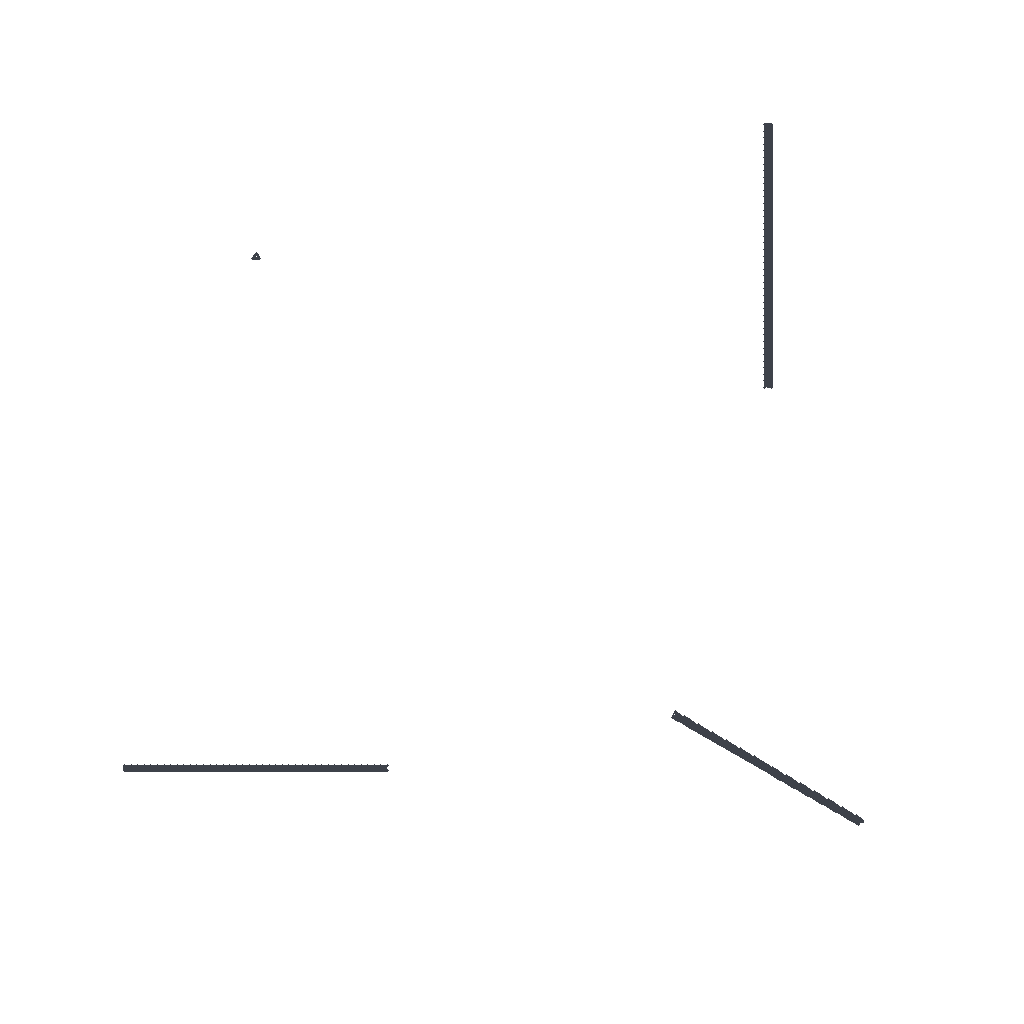Simulation study | abaqus
Set-up summary:
category,name,step,type,value,unit,region
solver,abaqus
solver,version,,,Abaqus/Standard 6.13-1
units,not stated in the deck,,not stated
analysis,deck,,modal,modal
load_step,Step-1,Step-1,modal
load_step,Step-2,Step-2,mode-based dynamic
load_step,requested,,,2
mesh,nodes,,,123
mesh,elements,,,480
element_type,T3D2,,truss,480
load,load commands in deck,,count,1
bc,support commands in deck,,count,3
material,MAT-TI,,in results
check,setup vs results,,match,"per instance, exact: element labels, types and connectivity; labels of the nodes the elements use; coordinates of those nodes at SINGLE_PRECISION in 1 of 1 instance(s)"
Abaqus input file, long lists of numbers shortened:
*Heading
** Job name: Job-ModalDynamics Model name: Model-1
** Generated by: Abaqus/CAE 6.13-1
*Preprint, echo=NO, model=NO, history=NO, contact=NO
**
** PARTS
**
*Part, name=Part-2
*Node
      1,           0.,          0.5,           0.
      2,           0.,           0.,           0.
** (121 more lines like these left out)
*Element, type=T3D2
1, 1, 2
2,  2, 83
** (478 more lines like these left out)
*Elset, elset=_PickedSet2, internal, generate
   1,  480,    1
** Section: Sect-Ti
*Solid Section, elset=_PickedSet2, material=Mat-Ti
0.0001,
*End Part
**
**
** ASSEMBLY
**
*Assembly, name=Assembly
**
*Instance, name=Part-2-1, part=Part-2
*End Instance
**
*Node
      1,         0.25,          20.,  0.144
*Nset, nset=Set-RP
 1,
*Nset, nset=_PickedSet485, internal, instance=Part-2-1, generate
  41,  123,   41
*Nset, nset=_PickedSet486, internal
 1,
*Nset, nset=_PickedSet488, internal, instance=Part-2-1, generate
  2,  84,  41
*Surface, type=NODE, name=_PickedSet485_CNS_, internal
_PickedSet485, 1.
** Constraint: Constraint-1
*MPC
PIN, _PickedSet485, _PickedSet486
*End Assembly
*Amplitude, name=Amp-1
             0.,              0.,            0.01,             0.1,            0.02,              1.,            0.98,              1.
           0.99,             0.1,              1.,              0.,             20.,              0.
**
** MATERIALS
**
*Material, name=Mat-Ti
*Density
4300.,
*Elastic
 1.06e+11, 0.3
**
** BOUNDARY CONDITIONS
**
** Name: BC-1 Type: Displacement/Rotation
*Boundary
_PickedSet488, 1, 1
_PickedSet488, 2, 2
_PickedSet488, 3, 3
** ----------------------------------------------------------------
**
** STEP: Step-1
**
*Step, name=Step-1, nlgeom=NO, perturbation
*Frequency, eigensolver=Lanczos, acoustic coupling=on, normalization=displacement
30, , , , ,
**
** OUTPUT REQUESTS
**
*Restart, write, frequency=0
**
** FIELD OUTPUT: F-Output-1
**
*Output, field, variable=PRESELECT
*End Step
** ----------------------------------------------------------------
**
** STEP: Step-2
**
*Step, name=Step-2, nlgeom=NO, perturbation
*Modal Dynamic, continue=NO
0.005, 20.
*Modal Damping
1, 30, 0.05
**
** LOADS
**
** Name: Load-1   Type: Concentrated force
*Cload, amplitude=Amp-1
Set-RP, 3, 100.
**
** OUTPUT REQUESTS
**
**
** FIELD OUTPUT: F-Output-2
**
*Output, field, frequency=1
*Node Output
A, U, V
*Element Output, directions=YES
E, S
**
** HISTORY OUTPUT: H-Output-1
**
*Output, history, frequency=1
*Node Output, nset=Set-RP
A3, U3, V3
*End Step
Results summary:
result,step,Step-1,partial,increments=0 time=0.0/1e-36
result,step,Step-2,partial,increments=0 time=0.0/20.0
result,analysis,,,mode-based dynamic
result,last_loadstep,,,2
result,primary field,,,U